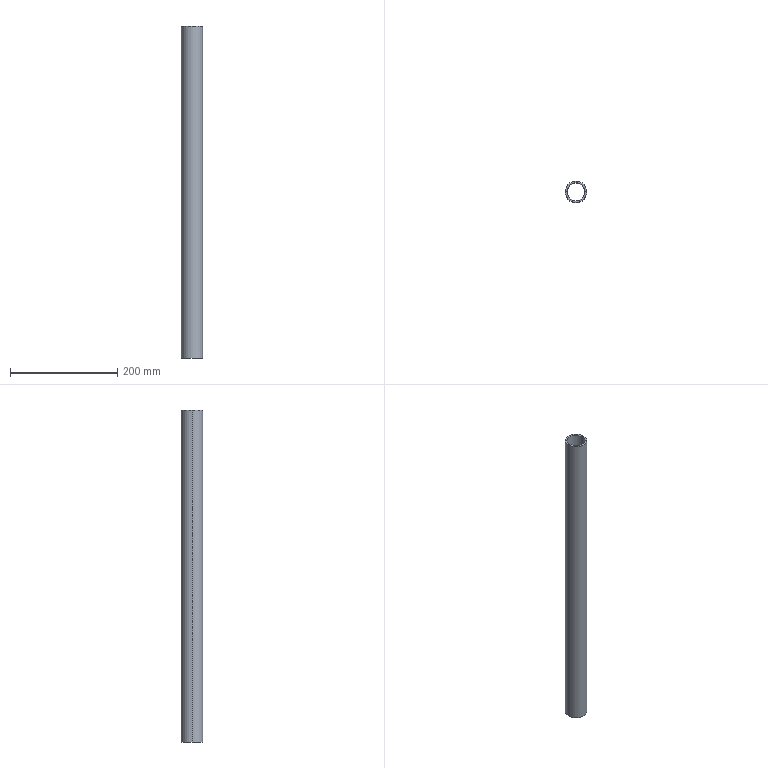Part | SolidWorks | features Extrusion 1, Shell 1 | 1 solid | 6 faces | box 40 x 40 x 618 mm | volume 228632 mm3 | cylinder 4 | plane 2 | commonest cylinder face diameters 33.6 x2 40 x2
STEP:
#1=CARTESIAN_POINT('',(-16.8,0.,618.));
#2=VERTEX_POINT('',#1);
#3=CARTESIAN_POINT('',(16.8,0.,618.));
#4=VERTEX_POINT('',#3);
#5=CARTESIAN_POINT('',(0.,0.,618.));
#6=DIRECTION('',(0.,0.,1.));
#7=DIRECTION('',(1.,0.,0.));
#8=AXIS2_PLACEMENT_3D('',#5,#6,#7);
#9=CIRCLE('',#8,16.8);
#10=EDGE_CURVE('',#2,#4,#9,.T.);
#11=ORIENTED_EDGE('',*,*,#10,.T.);
#12=CARTESIAN_POINT('',(16.8,0.,0.));
#13=VERTEX_POINT('',#12);
#14=CARTESIAN_POINT('',(16.8,0.,618.));
#15=DIRECTION('',(0.,0.,-1.));
#16=VECTOR('',#15,1000.);
#17=LINE('',#14,#16);
#18=EDGE_CURVE('',#4,#13,#17,.T.);
#19=ORIENTED_EDGE('',*,*,#18,.T.);
#20=CARTESIAN_POINT('',(-16.8,0.,0.));
#21=VERTEX_POINT('',#20);
#22=CARTESIAN_POINT('',(0.,0.,0.));
#23=DIRECTION('',(0.,0.,1.));
#24=DIRECTION('',(1.,0.,0.));
#25=AXIS2_PLACEMENT_3D('',#22,#23,#24);
#26=CIRCLE('',#25,16.8);
#27=EDGE_CURVE('',#21,#13,#26,.T.);
#28=ORIENTED_EDGE('',*,*,#27,.F.);
#29=CARTESIAN_POINT('',(-16.8,0.,618.));
#30=DIRECTION('',(0.,0.,-1.));
#31=VECTOR('',#30,1000.);
#32=LINE('',#29,#31);
#33=EDGE_CURVE('',#2,#21,#32,.T.);
#34=ORIENTED_EDGE('',*,*,#33,.F.);
#35=EDGE_LOOP('',(#11,#19,#28,#34));
#36=FACE_OUTER_BOUND('',#35,.T.);
#37=CARTESIAN_POINT('',(0.,0.,618.));
#38=DIRECTION('',(0.,0.,-1.));
#39=DIRECTION('',(-1.,0.,0.));
#40=AXIS2_PLACEMENT_3D('',#37,#38,#39);
#41=CYLINDRICAL_SURFACE('',#40,16.8);
#42=ADVANCED_FACE('',(#36),#41,.F.);
#43=CARTESIAN_POINT('',(20.,0.,618.));
#44=VERTEX_POINT('',#43);
#45=CARTESIAN_POINT('',(-20.,0.,618.));
#46=VERTEX_POINT('',#45);
#47=CARTESIAN_POINT('',(0.,0.,618.));
#48=DIRECTION('',(0.,0.,1.));
#49=DIRECTION('',(1.,0.,0.));
#50=AXIS2_PLACEMENT_3D('',#47,#48,#49);
#51=CIRCLE('',#50,20.);
#52=EDGE_CURVE('',#44,#46,#51,.T.);
#53=ORIENTED_EDGE('',*,*,#52,.F.);
#54=CARTESIAN_POINT('',(20.,0.,0.));
#55=VERTEX_POINT('',#54);
#56=CARTESIAN_POINT('',(20.,0.,618.));
#57=DIRECTION('',(0.,0.,-1.));
#58=VECTOR('',#57,1000.);
#59=LINE('',#56,#58);
#60=EDGE_CURVE('',#44,#55,#59,.T.);
#61=ORIENTED_EDGE('',*,*,#60,.T.);
#62=CARTESIAN_POINT('',(-20.,0.,0.));
#63=VERTEX_POINT('',#62);
#64=CARTESIAN_POINT('',(0.,0.,0.));
#65=DIRECTION('',(0.,0.,1.));
#66=DIRECTION('',(1.,0.,0.));
#67=AXIS2_PLACEMENT_3D('',#64,#65,#66);
#68=CIRCLE('',#67,20.);
#69=EDGE_CURVE('',#55,#63,#68,.T.);
#70=ORIENTED_EDGE('',*,*,#69,.T.);
#71=CARTESIAN_POINT('',(-20.,0.,618.));
#72=DIRECTION('',(0.,0.,-1.));
#73=VECTOR('',#72,1000.);
#74=LINE('',#71,#73);
#75=EDGE_CURVE('',#46,#63,#74,.T.);
#76=ORIENTED_EDGE('',*,*,#75,.F.);
#77=EDGE_LOOP('',(#53,#61,#70,#76));
#78=FACE_OUTER_BOUND('',#77,.T.);
#79=CARTESIAN_POINT('',(0.,0.,618.));
#80=DIRECTION('',(0.,0.,-1.));
#81=DIRECTION('',(-1.,0.,0.));
#82=AXIS2_PLACEMENT_3D('',#79,#80,#81);
#83=CYLINDRICAL_SURFACE('',#82,20.);
#84=ADVANCED_FACE('',(#78),#83,.T.);
#85=ORIENTED_EDGE('',*,*,#60,.F.);
#86=CARTESIAN_POINT('',(0.,0.,618.));
#87=DIRECTION('',(0.,0.,1.));
#88=DIRECTION('',(1.,0.,0.));
#89=AXIS2_PLACEMENT_3D('',#86,#87,#88);
#90=CIRCLE('',#89,20.);
#91=EDGE_CURVE('',#46,#44,#90,.T.);
#92=ORIENTED_EDGE('',*,*,#91,.F.);
#93=ORIENTED_EDGE('',*,*,#75,.T.);
#94=CARTESIAN_POINT('',(0.,0.,0.));
#95=DIRECTION('',(0.,0.,1.));
#96=DIRECTION('',(1.,0.,0.));
#97=AXIS2_PLACEMENT_3D('',#94,#95,#96);
#98=CIRCLE('',#97,20.);
#99=EDGE_CURVE('',#63,#55,#98,.T.);
#100=ORIENTED_EDGE('',*,*,#99,.T.);
#101=EDGE_LOOP('',(#85,#92,#93,#100));
#102=FACE_OUTER_BOUND('',#101,.T.);
#103=CARTESIAN_POINT('',(0.,0.,618.));
#104=DIRECTION('',(0.,0.,-1.));
#105=DIRECTION('',(-1.,0.,0.));
#106=AXIS2_PLACEMENT_3D('',#103,#104,#105);
#107=CYLINDRICAL_SURFACE('',#106,20.);
#108=ADVANCED_FACE('',(#102),#107,.T.);
#109=ORIENTED_EDGE('',*,*,#10,.F.);
#110=CARTESIAN_POINT('',(0.,0.,618.));
#111=DIRECTION('',(0.,0.,1.));
#112=DIRECTION('',(1.,0.,0.));
#113=AXIS2_PLACEMENT_3D('',#110,#111,#112);
#114=CIRCLE('',#113,16.8);
#115=EDGE_CURVE('',#4,#2,#114,.T.);
#116=ORIENTED_EDGE('',*,*,#115,.F.);
#117=EDGE_LOOP('',(#109,#116));
#118=FACE_BOUND('',#117,.T.);
#119=ORIENTED_EDGE('',*,*,#91,.T.);
#120=ORIENTED_EDGE('',*,*,#52,.T.);
#121=EDGE_LOOP('',(#119,#120));
#122=FACE_OUTER_BOUND('',#121,.T.);
#123=CARTESIAN_POINT('',(0.,0.,618.));
#124=DIRECTION('',(0.,0.,1.));
#125=DIRECTION('',(1.,0.,0.));
#126=AXIS2_PLACEMENT_3D('',#123,#124,#125);
#127=PLANE('',#126);
#128=ADVANCED_FACE('',(#118,#122),#127,.T.);
#129=ORIENTED_EDGE('',*,*,#27,.T.);
#130=CARTESIAN_POINT('',(0.,0.,0.));
#131=DIRECTION('',(0.,0.,1.));
#132=DIRECTION('',(1.,0.,0.));
#133=AXIS2_PLACEMENT_3D('',#130,#131,#132);
#134=CIRCLE('',#133,16.8);
#135=EDGE_CURVE('',#13,#21,#134,.T.);
#136=ORIENTED_EDGE('',*,*,#135,.T.);
#137=EDGE_LOOP('',(#129,#136));
#138=FACE_BOUND('',#137,.T.);
#139=ORIENTED_EDGE('',*,*,#99,.F.);
#140=ORIENTED_EDGE('',*,*,#69,.F.);
#141=EDGE_LOOP('',(#139,#140));
#142=FACE_OUTER_BOUND('',#141,.T.);
#143=CARTESIAN_POINT('',(0.,0.,0.));
#144=DIRECTION('',(0.,0.,1.));
#145=DIRECTION('',(1.,0.,0.));
#146=AXIS2_PLACEMENT_3D('',#143,#144,#145);
#147=PLANE('',#146);
#148=ADVANCED_FACE('',(#138,#142),#147,.F.);
#149=ORIENTED_EDGE('',*,*,#18,.F.);
#150=ORIENTED_EDGE('',*,*,#115,.T.);
#151=ORIENTED_EDGE('',*,*,#33,.T.);
#152=ORIENTED_EDGE('',*,*,#135,.F.);
#153=EDGE_LOOP('',(#149,#150,#151,#152));
#154=FACE_OUTER_BOUND('',#153,.T.);
#155=CARTESIAN_POINT('',(0.,0.,618.));
#156=DIRECTION('',(0.,0.,-1.));
#157=DIRECTION('',(-1.,0.,0.));
#158=AXIS2_PLACEMENT_3D('',#155,#156,#157);
#159=CYLINDRICAL_SURFACE('',#158,16.8);
#160=ADVANCED_FACE('',(#154),#159,.F.);
#161=CLOSED_SHELL('',(#42,#84,#108,#128,#148,#160));
#162=MANIFOLD_SOLID_BREP('',#161);
#163=CARTESIAN_POINT('',(0.,0.,0.));
#164=DIRECTION('',(0.,0.,1.));
#165=DIRECTION('',(1.,0.,0.));
#166=AXIS2_PLACEMENT_3D('',#163,#164,#165);
#167=(LENGTH_UNIT()NAMED_UNIT(*)SI_UNIT(.MILLI.,.METRE.));
#168=UNCERTAINTY_MEASURE_WITH_UNIT(LENGTH_MEASURE(0.00001),#167,'','');
#169=(NAMED_UNIT(*)PLANE_ANGLE_UNIT()SI_UNIT($,.RADIAN.));
#170=(NAMED_UNIT(*)SI_UNIT($,.STERADIAN.)SOLID_ANGLE_UNIT());
#171=(GEOMETRIC_REPRESENTATION_CONTEXT(3)GLOBAL_UNCERTAINTY_ASSIGNED_CONTEXT((#168))GLOBAL_UNIT_ASSIGNED_CONTEXT((#167,#169,#170))REPRESENTATION_CONTEXT('',''));
#172=ADVANCED_BREP_SHAPE_REPRESENTATION('',(#162,#166),#171);